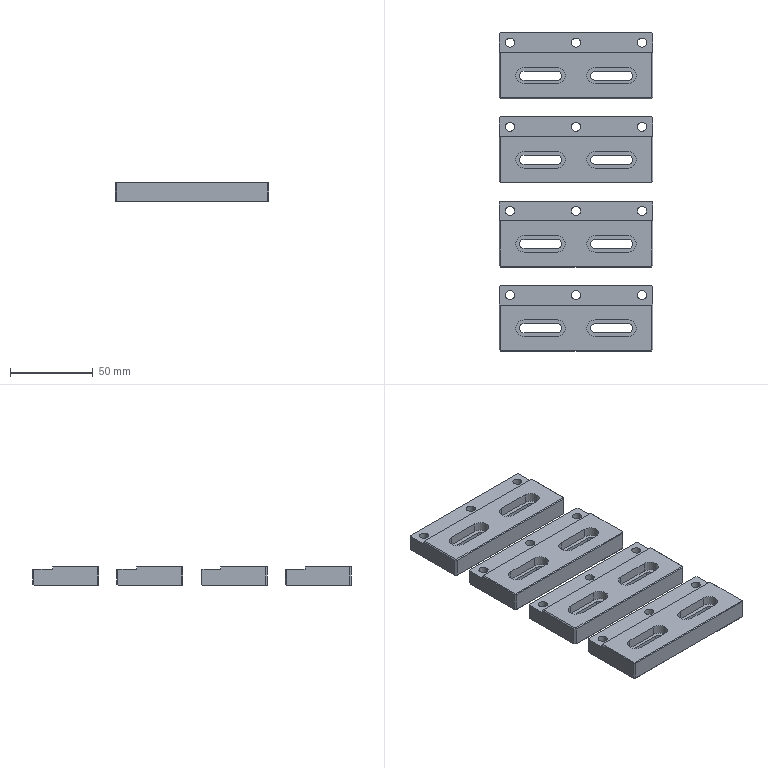Part | 4 solids | 208 faces | box 93.002 x 193 x 12 mm | volume 143193 mm3 | plane 152 | cylinder 56 | commonest cylinder face diameters 5.5 x28 10 x28